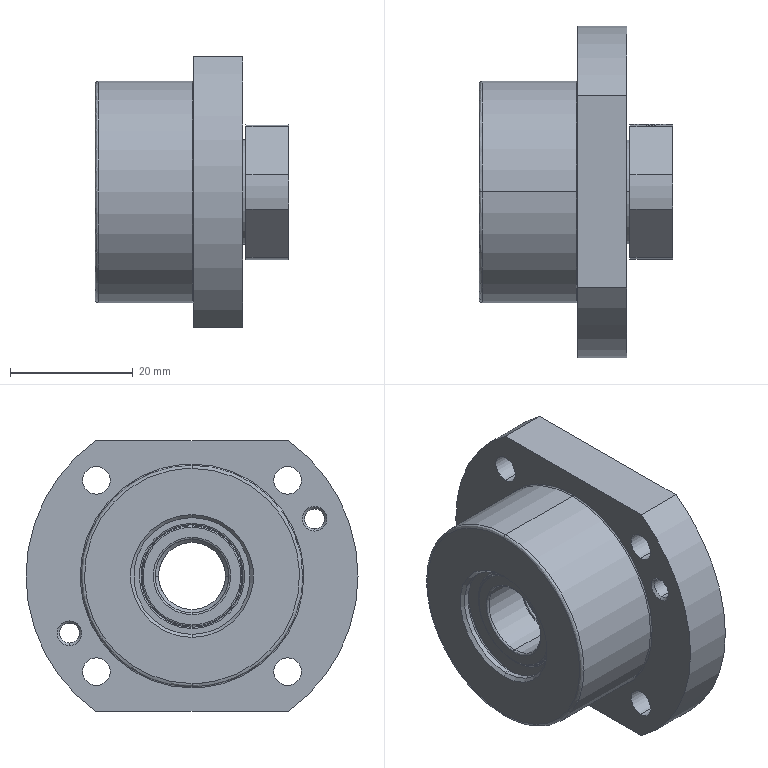Part | SolidWorks | 6 solids | 393 faces | box 31.5 x 54 x 44 mm | volume 27401 mm3 | cylinder 127 | cone 104 | spline 102 | plane 60 | commonest cylinder face diameters 2.1 x8 4.5 x8 8 x8 15.5 x8 16.3 x8 16.7 x8